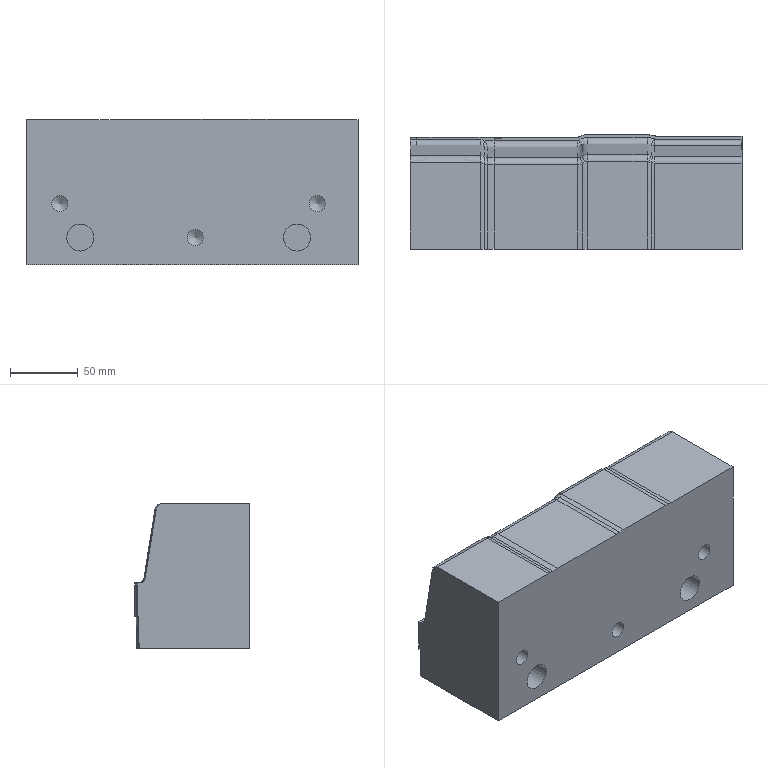Part | NX | features solid 2 | 1 solid | 68 faces | box 245 x 84.549 x 107.259 mm | volume 1984457 mm3 | spline 28 | cylinder 20 | plane 17 | cone 3 | commonest cylinder face diameters 10 x8 12 x5 8 x3 14 x2 20 x2